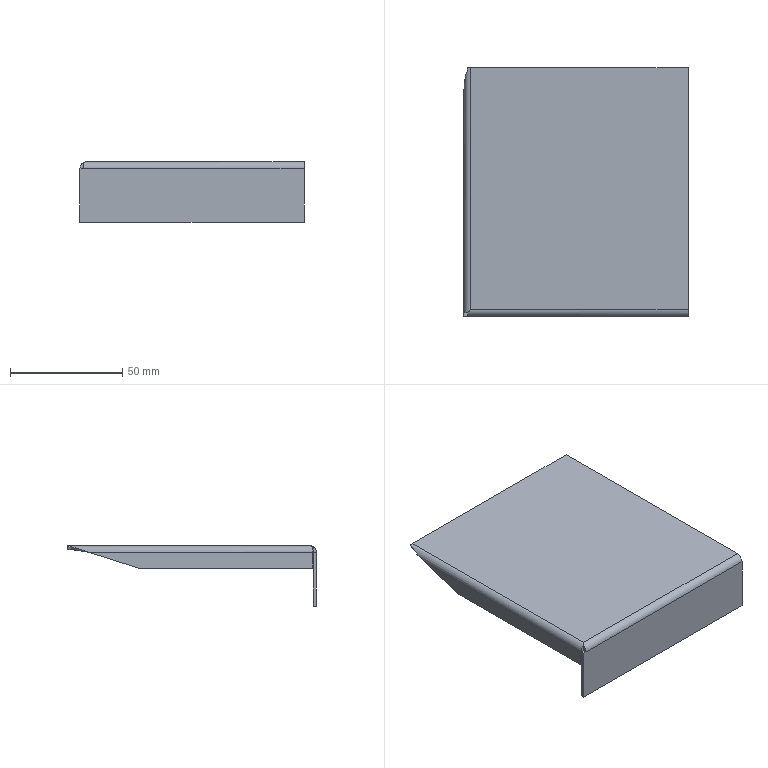Part | NX | features solid 2 | 1 solid | 23 faces | box 100 x 111 x 27 mm | volume 21325 mm3 | plane 18 | cylinder 4 | spline 1 | commonest cylinder face diameters 3 x2 6 x2
STEP:
#1=CARTESIAN_POINT('',(473.5,-28.4,8.5));
#2=VERTEX_POINT('',#1);
#3=CARTESIAN_POINT('',(473.5,71.235,8.5));
#4=VERTEX_POINT('',#3);
#5=CARTESIAN_POINT('',(473.5,-30.,8.5));
#6=DIRECTION('',(0.,1.,0.));
#7=VECTOR('',#6,1000.);
#8=LINE('',#5,#7);
#9=EDGE_CURVE('',#2,#4,#8,.T.);
#10=ORIENTED_EDGE('',*,*,#9,.T.);
#11=CARTESIAN_POINT('',(473.5,49.36,1.5));
#12=VERTEX_POINT('',#11);
#13=CARTESIAN_POINT('',(473.5,-19.726,-20.607));
#14=DIRECTION('',(0.,0.9524,0.3048));
#15=VECTOR('',#14,1000.);
#16=LINE('',#13,#15);
#17=EDGE_CURVE('',#12,#4,#16,.T.);
#18=ORIENTED_EDGE('',*,*,#17,.F.);
#19=CARTESIAN_POINT('',(473.5,-28.4,1.5));
#20=VERTEX_POINT('',#19);
#21=CARTESIAN_POINT('',(473.5,-30.,1.5));
#22=DIRECTION('',(0.,1.,0.));
#23=VECTOR('',#22,1000.);
#24=LINE('',#21,#23);
#25=EDGE_CURVE('',#20,#12,#24,.T.);
#26=ORIENTED_EDGE('',*,*,#25,.F.);
#27=CARTESIAN_POINT('',(473.5,-28.4,11.5));
#28=DIRECTION('',(0.,0.,-1.));
#29=VECTOR('',#28,1000.);
#30=LINE('',#27,#29);
#31=EDGE_CURVE('',#2,#20,#30,.T.);
#32=ORIENTED_EDGE('',*,*,#31,.F.);
#33=EDGE_LOOP('',(#10,#18,#26,#32));
#34=FACE_BOUND('',#33,.T.);
#35=CARTESIAN_POINT('',(473.5,-30.,11.5));
#36=DIRECTION('',(1.,0.,0.));
#37=DIRECTION('',(0.,1.,0.));
#38=AXIS2_PLACEMENT_3D('',#35,#36,#37);
#39=PLANE('',#38);
#40=ADVANCED_FACE('',(#34),#39,.F.);
#41=CARTESIAN_POINT('',(475.,49.36,1.5));
#42=VERTEX_POINT('',#41);
#43=CARTESIAN_POINT('',(475.,71.235,8.5));
#44=VERTEX_POINT('',#43);
#45=CARTESIAN_POINT('',(475.,-19.726,-20.607));
#46=DIRECTION('',(0.,0.9524,0.3048));
#47=VECTOR('',#46,1000.);
#48=LINE('',#45,#47);
#49=EDGE_CURVE('',#42,#44,#48,.T.);
#50=ORIENTED_EDGE('',*,*,#49,.T.);
#51=CARTESIAN_POINT('',(475.,-28.4,8.5));
#52=VERTEX_POINT('',#51);
#53=CARTESIAN_POINT('',(475.,-30.,8.5));
#54=DIRECTION('',(0.,1.,0.));
#55=VECTOR('',#54,1000.);
#56=LINE('',#53,#55);
#57=EDGE_CURVE('',#52,#44,#56,.T.);
#58=ORIENTED_EDGE('',*,*,#57,.F.);
#59=CARTESIAN_POINT('',(475.,-28.4,1.5));
#60=VERTEX_POINT('',#59);
#61=CARTESIAN_POINT('',(475.,-28.4,11.5));
#62=DIRECTION('',(0.,0.,-1.));
#63=VECTOR('',#62,1000.);
#64=LINE('',#61,#63);
#65=EDGE_CURVE('',#52,#60,#64,.T.);
#66=ORIENTED_EDGE('',*,*,#65,.T.);
#67=CARTESIAN_POINT('',(475.,-30.,1.5));
#68=DIRECTION('',(0.,1.,0.));
#69=VECTOR('',#68,1000.);
#70=LINE('',#67,#69);
#71=EDGE_CURVE('',#60,#42,#70,.T.);
#72=ORIENTED_EDGE('',*,*,#71,.T.);
#73=EDGE_LOOP('',(#50,#58,#66,#72));
#74=FACE_BOUND('',#73,.T.);
#75=CARTESIAN_POINT('',(475.,-30.,11.5));
#76=DIRECTION('',(1.,0.,0.));
#77=DIRECTION('',(0.,1.,0.));
#78=AXIS2_PLACEMENT_3D('',#75,#76,#77);
#79=PLANE('',#78);
#80=ADVANCED_FACE('',(#74),#79,.T.);
#81=CARTESIAN_POINT('',(473.5,49.36,1.5));
#82=DIRECTION('',(-1.,0.,0.));
#83=VECTOR('',#82,1000.);
#84=LINE('',#81,#83);
#85=EDGE_CURVE('',#42,#12,#84,.T.);
#86=ORIENTED_EDGE('',*,*,#85,.T.);
#87=ORIENTED_EDGE('',*,*,#17,.T.);
#88=CARTESIAN_POINT('',(473.5,71.235,8.5));
#89=DIRECTION('',(-1.,0.,0.));
#90=VECTOR('',#89,1000.);
#91=LINE('',#88,#90);
#92=EDGE_CURVE('',#44,#4,#91,.T.);
#93=ORIENTED_EDGE('',*,*,#92,.F.);
#94=ORIENTED_EDGE('',*,*,#49,.F.);
#95=EDGE_LOOP('',(#86,#87,#93,#94));
#96=FACE_BOUND('',#95,.T.);
#97=CARTESIAN_POINT('',(473.5,-19.726,-20.607));
#98=DIRECTION('',(0.,0.3048,-0.9524));
#99=DIRECTION('',(-1.,0.,0.));
#100=AXIS2_PLACEMENT_3D('',#97,#98,#99);
#101=PLANE('',#100);
#102=ADVANCED_FACE('',(#96),#101,.T.);
#103=ORIENTED_EDGE('',*,*,#85,.F.);
#104=ORIENTED_EDGE('',*,*,#71,.F.);
#105=CARTESIAN_POINT('',(473.5,-28.4,1.5));
#106=DIRECTION('',(-1.,0.,0.));
#107=VECTOR('',#106,1000.);
#108=LINE('',#105,#107);
#109=EDGE_CURVE('',#60,#20,#108,.T.);
#110=ORIENTED_EDGE('',*,*,#109,.T.);
#111=ORIENTED_EDGE('',*,*,#25,.T.);
#112=EDGE_LOOP('',(#103,#104,#110,#111));
#113=FACE_BOUND('',#112,.T.);
#114=CARTESIAN_POINT('',(473.5,-30.,1.5));
#115=DIRECTION('',(0.,0.,-1.));
#116=DIRECTION('',(0.,-1.,0.));
#117=AXIS2_PLACEMENT_3D('',#114,#115,#116);
#118=PLANE('',#117);
#119=ADVANCED_FACE('',(#113),#118,.T.);
#120=CARTESIAN_POINT('',(476.5,-27.,10.));
#121=VERTEX_POINT('',#120);
#122=CARTESIAN_POINT('',(573.5,-27.,10.));
#123=VERTEX_POINT('',#122);
#124=CARTESIAN_POINT('',(476.5,-27.,10.));
#125=DIRECTION('',(1.,0.,0.));
#126=VECTOR('',#125,1000.);
#127=LINE('',#124,#126);
#128=EDGE_CURVE('',#121,#123,#127,.T.);
#129=ORIENTED_EDGE('',*,*,#128,.F.);
#130=CARTESIAN_POINT('',(476.5,81.,10.));
#131=VERTEX_POINT('',#130);
#132=CARTESIAN_POINT('',(476.5,-30.,10.));
#133=DIRECTION('',(0.,1.,0.));
#134=VECTOR('',#133,1000.);
#135=LINE('',#132,#134);
#136=EDGE_CURVE('',#121,#131,#135,.T.);
#137=ORIENTED_EDGE('',*,*,#136,.T.);
#138=CARTESIAN_POINT('',(573.5,81.,10.));
#139=VERTEX_POINT('',#138);
#140=CARTESIAN_POINT('',(573.5,81.,10.));
#141=DIRECTION('',(-1.,0.,0.));
#142=VECTOR('',#141,1000.);
#143=LINE('',#140,#142);
#144=EDGE_CURVE('',#139,#131,#143,.T.);
#145=ORIENTED_EDGE('',*,*,#144,.F.);
#146=CARTESIAN_POINT('',(573.5,-30.,10.));
#147=DIRECTION('',(0.,1.,0.));
#148=VECTOR('',#147,1000.);
#149=LINE('',#146,#148);
#150=EDGE_CURVE('',#123,#139,#149,.T.);
#151=ORIENTED_EDGE('',*,*,#150,.F.);
#152=EDGE_LOOP('',(#129,#137,#145,#151));
#153=FACE_BOUND('',#152,.T.);
#154=CARTESIAN_POINT('',(573.5,-30.,10.));
#155=DIRECTION('',(0.,0.,-1.));
#156=DIRECTION('',(0.,-1.,0.));
#157=AXIS2_PLACEMENT_3D('',#154,#155,#156);
#158=PLANE('',#157);
#159=ADVANCED_FACE('',(#153),#158,.T.);
#160=CARTESIAN_POINT('',(476.5,-27.,11.5));
#161=VERTEX_POINT('',#160);
#162=CARTESIAN_POINT('',(476.5,81.,11.5));
#163=VERTEX_POINT('',#162);
#164=CARTESIAN_POINT('',(476.5,-30.,11.5));
#165=DIRECTION('',(0.,1.,0.));
#166=VECTOR('',#165,1000.);
#167=LINE('',#164,#166);
#168=EDGE_CURVE('',#161,#163,#167,.T.);
#169=ORIENTED_EDGE('',*,*,#168,.F.);
#170=CARTESIAN_POINT('',(573.5,-27.,11.5));
#171=VERTEX_POINT('',#170);
#172=CARTESIAN_POINT('',(476.5,-27.,11.5));
#173=DIRECTION('',(1.,0.,0.));
#174=VECTOR('',#173,1000.);
#175=LINE('',#172,#174);
#176=EDGE_CURVE('',#161,#171,#175,.T.);
#177=ORIENTED_EDGE('',*,*,#176,.T.);
#178=CARTESIAN_POINT('',(573.5,81.,11.5));
#179=VERTEX_POINT('',#178);
#180=CARTESIAN_POINT('',(573.5,-30.,11.5));
#181=DIRECTION('',(0.,1.,0.));
#182=VECTOR('',#181,1000.);
#183=LINE('',#180,#182);
#184=EDGE_CURVE('',#171,#179,#183,.T.);
#185=ORIENTED_EDGE('',*,*,#184,.T.);
#186=CARTESIAN_POINT('',(573.5,81.,11.5));
#187=DIRECTION('',(-1.,0.,0.));
#188=VECTOR('',#187,1000.);
#189=LINE('',#186,#188);
#190=EDGE_CURVE('',#179,#163,#189,.T.);
#191=ORIENTED_EDGE('',*,*,#190,.T.);
#192=EDGE_LOOP('',(#169,#177,#185,#191));
#193=FACE_BOUND('',#192,.T.);
#194=CARTESIAN_POINT('',(573.5,-30.,11.5));
#195=DIRECTION('',(0.,0.,-1.));
#196=DIRECTION('',(0.,-1.,0.));
#197=AXIS2_PLACEMENT_3D('',#194,#195,#196);
#198=PLANE('',#197);
#199=ADVANCED_FACE('',(#193),#198,.F.);
#200=CARTESIAN_POINT('',(475.1,-30.,8.5));
#201=VERTEX_POINT('',#200);
#202=CARTESIAN_POINT('',(475.1,-28.5,8.5));
#203=VERTEX_POINT('',#202);
#204=CARTESIAN_POINT('',(475.1,-30.,8.5));
#205=DIRECTION('',(0.,1.,0.));
#206=VECTOR('',#205,1000.);
#207=LINE('',#204,#206);
#208=EDGE_CURVE('',#201,#203,#207,.T.);
#209=ORIENTED_EDGE('',*,*,#208,.F.);
#210=CARTESIAN_POINT('',(475.1,-28.5,11.098));
#211=VERTEX_POINT('',#210);
#212=CARTESIAN_POINT('',(475.1,-27.,8.5));
#213=DIRECTION('',(-1.,0.,0.));
#214=DIRECTION('',(0.,0.,1.));
#215=AXIS2_PLACEMENT_3D('',#212,#213,#214);
#216=CIRCLE('',#215,3.);
#217=EDGE_CURVE('',#201,#211,#216,.T.);
#218=ORIENTED_EDGE('',*,*,#217,.T.);
#219=CARTESIAN_POINT('',(475.1,-28.5,-988.5));
#220=DIRECTION('',(0.,0.,-1.));
#221=VECTOR('',#220,1000.);
#222=LINE('',#219,#221);
#223=EDGE_CURVE('',#211,#203,#222,.T.);
#224=ORIENTED_EDGE('',*,*,#223,.T.);
#225=EDGE_LOOP('',(#209,#218,#224));
#226=FACE_BOUND('',#225,.T.);
#227=CARTESIAN_POINT('',(475.1,-28.5,1011.5));
#228=DIRECTION('',(1.,0.,0.));
#229=DIRECTION('',(0.,1.,0.));
#230=AXIS2_PLACEMENT_3D('',#227,#228,#229);
#231=PLANE('',#230);
#232=ADVANCED_FACE('',(#226),#231,.F.);
#233=CARTESIAN_POINT('',(475.1,-28.5,8.5));
#234=CARTESIAN_POINT('',(475.1,-28.5,9.379));
#235=CARTESIAN_POINT('',(475.68,-27.879,10.));
#236=CARTESIAN_POINT('',(476.5,-27.,10.));
#237=(BOUNDED_CURVE()B_SPLINE_CURVE(3,(#233,#234,#235,#236),.UNSPECIFIED.,.F.,.F.)B_SPLINE_CURVE_WITH_KNOTS((4,4),(3.142,4.712),.PIECEWISE_BEZIER_KNOTS.)CURVE()GEOMETRIC_REPRESENTATION_ITEM()RATIONAL_B_SPLINE_CURVE((1.,0.8047,0.8047,1.))REPRESENTATION_ITEM(''));
#238=EDGE_CURVE('',#203,#121,#237,.T.);
#239=ORIENTED_EDGE('',*,*,#238,.F.);
#240=ORIENTED_EDGE('',*,*,#223,.F.);
#241=CARTESIAN_POINT('',(475.1,-28.5,11.098));
#242=CARTESIAN_POINT('',(475.528,-28.041,11.363));
#243=CARTESIAN_POINT('',(476.006,-27.53,11.5));
#244=CARTESIAN_POINT('',(476.5,-27.,11.5));
#245=(BOUNDED_CURVE()B_SPLINE_CURVE(3,(#241,#242,#243,#244),.UNSPECIFIED.,.F.,.F.)B_SPLINE_CURVE_WITH_KNOTS((4,4),(4.189,4.712),.PIECEWISE_BEZIER_KNOTS.)CURVE()GEOMETRIC_REPRESENTATION_ITEM()RATIONAL_B_SPLINE_CURVE((1.,0.9773,0.9773,1.))REPRESENTATION_ITEM(''));
#246=EDGE_CURVE('',#211,#161,#245,.T.);
#247=ORIENTED_EDGE('',*,*,#246,.T.);
#248=CARTESIAN_POINT('',(476.5,-27.,10.));
#249=DIRECTION('',(0.,0.,1.));
#250=VECTOR('',#249,1000.);
#251=LINE('',#248,#250);
#252=EDGE_CURVE('',#121,#161,#251,.T.);
#253=ORIENTED_EDGE('',*,*,#252,.F.);
#254=EDGE_LOOP('',(#239,#240,#247,#253));
#255=FACE_BOUND('',#254,.T.);
#256=CARTESIAN_POINT('',(1158.818,704.055,1011.5));
#257=DIRECTION('',(0.7311,-0.6823,0.));
#258=DIRECTION('',(0.,0.,-1.));
#259=AXIS2_PLACEMENT_3D('',#256,#257,#258);
#260=PLANE('',#259);
#261=ADVANCED_FACE('',(#255),#260,.F.);
#262=ORIENTED_EDGE('',*,*,#246,.F.);
#263=ORIENTED_EDGE('',*,*,#217,.F.);
#264=CARTESIAN_POINT('',(573.5,-30.,8.5));
#265=VERTEX_POINT('',#264);
#266=CARTESIAN_POINT('',(573.5,-30.,8.5));
#267=DIRECTION('',(-1.,0.,0.));
#268=VECTOR('',#267,1000.);
#269=LINE('',#266,#268);
#270=EDGE_CURVE('',#265,#201,#269,.T.);
#271=ORIENTED_EDGE('',*,*,#270,.F.);
#272=CARTESIAN_POINT('',(573.5,-27.,8.5));
#273=DIRECTION('',(-1.,0.,0.));
#274=DIRECTION('',(0.,0.,-1.));
#275=AXIS2_PLACEMENT_3D('',#272,#273,#274);
#276=CIRCLE('',#275,3.);
#277=EDGE_CURVE('',#265,#171,#276,.T.);
#278=ORIENTED_EDGE('',*,*,#277,.T.);
#279=ORIENTED_EDGE('',*,*,#176,.F.);
#280=EDGE_LOOP('',(#262,#263,#271,#278,#279));
#281=FACE_BOUND('',#280,.T.);
#282=CARTESIAN_POINT('',(476.5,-27.,8.5));
#283=DIRECTION('',(1.,0.,0.));
#284=DIRECTION('',(0.,0.,-1.));
#285=AXIS2_PLACEMENT_3D('',#282,#283,#284);
#286=CYLINDRICAL_SURFACE('',#285,3.);
#287=ADVANCED_FACE('',(#281),#286,.T.);
#288=ORIENTED_EDGE('',*,*,#277,.F.);
#289=CARTESIAN_POINT('',(573.5,-30.,-15.5));
#290=VERTEX_POINT('',#289);
#291=CARTESIAN_POINT('',(573.5,-30.,10.208));
#292=DIRECTION('',(0.,0.,1.));
#293=VECTOR('',#292,1000.);
#294=LINE('',#291,#293);
#295=EDGE_CURVE('',#290,#265,#294,.T.);
#296=ORIENTED_EDGE('',*,*,#295,.F.);
#297=CARTESIAN_POINT('',(573.5,-28.5,-15.5));
#298=VERTEX_POINT('',#297);
#299=CARTESIAN_POINT('',(573.5,-30.,-15.5));
#300=DIRECTION('',(0.,1.,0.));
#301=VECTOR('',#300,1000.);
#302=LINE('',#299,#301);
#303=EDGE_CURVE('',#290,#298,#302,.T.);
#304=ORIENTED_EDGE('',*,*,#303,.T.);
#305=CARTESIAN_POINT('',(573.5,-28.5,8.5));
#306=VERTEX_POINT('',#305);
#307=CARTESIAN_POINT('',(573.5,-28.5,10.208));
#308=DIRECTION('',(0.,0.,1.));
#309=VECTOR('',#308,1000.);
#310=LINE('',#307,#309);
#311=EDGE_CURVE('',#298,#306,#310,.T.);
#312=ORIENTED_EDGE('',*,*,#311,.T.);
#313=CARTESIAN_POINT('',(573.5,-27.,8.5));
#314=DIRECTION('',(-1.,0.,0.));
#315=DIRECTION('',(0.,0.,1.));
#316=AXIS2_PLACEMENT_3D('',#313,#314,#315);
#317=CIRCLE('',#316,1.5);
#318=EDGE_CURVE('',#306,#123,#317,.T.);
#319=ORIENTED_EDGE('',*,*,#318,.T.);
#320=ORIENTED_EDGE('',*,*,#150,.T.);
#321=CARTESIAN_POINT('',(573.5,81.,11.5));
#322=DIRECTION('',(0.,0.,1.));
#323=VECTOR('',#322,1000.);
#324=LINE('',#321,#323);
#325=EDGE_CURVE('',#139,#179,#324,.T.);
#326=ORIENTED_EDGE('',*,*,#325,.T.);
#327=ORIENTED_EDGE('',*,*,#184,.F.);
#328=EDGE_LOOP('',(#288,#296,#304,#312,#319,#320,#326,#327));
#329=FACE_BOUND('',#328,.T.);
#330=CARTESIAN_POINT('',(573.5,-30.,11.5));
#331=DIRECTION('',(-1.,0.,0.));
#332=DIRECTION('',(0.,1.,0.));
#333=AXIS2_PLACEMENT_3D('',#330,#331,#332);
#334=PLANE('',#333);
#335=ADVANCED_FACE('',(#329),#334,.F.);
#336=CARTESIAN_POINT('',(573.5,-28.5,8.5));
#337=DIRECTION('',(-1.,0.,0.));
#338=VECTOR('',#337,1000.);
#339=LINE('',#336,#338);
#340=EDGE_CURVE('',#306,#203,#339,.T.);
#341=ORIENTED_EDGE('',*,*,#340,.T.);
#342=ORIENTED_EDGE('',*,*,#238,.T.);
#343=ORIENTED_EDGE('',*,*,#128,.T.);
#344=ORIENTED_EDGE('',*,*,#318,.F.);
#345=EDGE_LOOP('',(#341,#342,#343,#344));
#346=FACE_BOUND('',#345,.T.);
#347=CARTESIAN_POINT('',(476.5,-27.,8.5));
#348=DIRECTION('',(1.,0.,0.));
#349=DIRECTION('',(0.,0.,-1.));
#350=AXIS2_PLACEMENT_3D('',#347,#348,#349);
#351=CYLINDRICAL_SURFACE('',#350,1.5);
#352=ADVANCED_FACE('',(#346),#351,.F.);
#353=CARTESIAN_POINT('',(476.5,-27.,10.));
#354=CARTESIAN_POINT('',(475.621,-27.82,10.));
#355=CARTESIAN_POINT('',(475.,-28.4,9.379));
#356=CARTESIAN_POINT('',(475.,-28.4,8.5));
#357=(BOUNDED_CURVE()B_SPLINE_CURVE(3,(#353,#354,#355,#356),.UNSPECIFIED.,.F.,.F.)B_SPLINE_CURVE_WITH_KNOTS((4,4),(1.571,3.142),.PIECEWISE_BEZIER_KNOTS.)CURVE()GEOMETRIC_REPRESENTATION_ITEM()RATIONAL_B_SPLINE_CURVE((1.,0.8047,0.8047,1.))REPRESENTATION_ITEM(''));
#358=EDGE_CURVE('',#121,#52,#357,.T.);
#359=ORIENTED_EDGE('',*,*,#358,.F.);
#360=ORIENTED_EDGE('',*,*,#252,.T.);
#361=CARTESIAN_POINT('',(475.,-28.4,11.098));
#362=VERTEX_POINT('',#361);
#363=CARTESIAN_POINT('',(476.5,-27.,11.5));
#364=CARTESIAN_POINT('',(475.97,-27.494,11.5));
#365=CARTESIAN_POINT('',(475.459,-27.972,11.363));
#366=CARTESIAN_POINT('',(475.,-28.4,11.098));
#367=(BOUNDED_CURVE()B_SPLINE_CURVE(3,(#363,#364,#365,#366),.UNSPECIFIED.,.F.,.F.)B_SPLINE_CURVE_WITH_KNOTS((4,4),(1.571,2.094),.PIECEWISE_BEZIER_KNOTS.)CURVE()GEOMETRIC_REPRESENTATION_ITEM()RATIONAL_B_SPLINE_CURVE((1.,0.9773,0.9773,1.))REPRESENTATION_ITEM(''));
#368=EDGE_CURVE('',#161,#362,#367,.T.);
#369=ORIENTED_EDGE('',*,*,#368,.T.);
#370=CARTESIAN_POINT('',(475.,-28.4,-988.5));
#371=DIRECTION('',(0.,0.,-1.));
#372=VECTOR('',#371,1000.);
#373=LINE('',#370,#372);
#374=EDGE_CURVE('',#362,#52,#373,.T.);
#375=ORIENTED_EDGE('',*,*,#374,.T.);
#376=EDGE_LOOP('',(#359,#360,#369,#375));
#377=FACE_BOUND('',#376,.T.);
#378=CARTESIAN_POINT('',(1207.555,655.318,1011.5));
#379=DIRECTION('',(0.6823,-0.7311,0.));
#380=DIRECTION('',(0.,0.,-1.));
#381=AXIS2_PLACEMENT_3D('',#378,#379,#380);
#382=PLANE('',#381);
#383=ADVANCED_FACE('',(#377),#382,.T.);
#384=CARTESIAN_POINT('',(476.5,-28.4,8.5));
#385=DIRECTION('',(0.,-1.,0.));
#386=DIRECTION('',(0.,0.,-1.));
#387=AXIS2_PLACEMENT_3D('',#384,#385,#386);
#388=CIRCLE('',#387,3.);
#389=EDGE_CURVE('',#362,#2,#388,.T.);
#390=ORIENTED_EDGE('',*,*,#389,.T.);
#391=ORIENTED_EDGE('',*,*,#31,.T.);
#392=ORIENTED_EDGE('',*,*,#109,.F.);
#393=ORIENTED_EDGE('',*,*,#65,.F.);
#394=ORIENTED_EDGE('',*,*,#374,.F.);
#395=EDGE_LOOP('',(#390,#391,#392,#393,#394));
#396=FACE_BOUND('',#395,.T.);
#397=CARTESIAN_POINT('',(475.,-28.4,1011.5));
#398=DIRECTION('',(0.,-1.,0.));
#399=DIRECTION('',(-1.,0.,0.));
#400=AXIS2_PLACEMENT_3D('',#397,#398,#399);
#401=PLANE('',#400);
#402=ADVANCED_FACE('',(#396),#401,.T.);
#403=CARTESIAN_POINT('',(475.75,81.,9.799));
#404=VERTEX_POINT('',#403);
#405=CARTESIAN_POINT('',(475.75,79.354,9.799));
#406=VERTEX_POINT('',#405);
#407=CARTESIAN_POINT('',(475.75,-30.,9.799));
#408=DIRECTION('',(0.,-1.,0.));
#409=VECTOR('',#408,1000.);
#410=LINE('',#407,#409);
#411=EDGE_CURVE('',#404,#406,#410,.T.);
#412=ORIENTED_EDGE('',*,*,#411,.T.);
#413=CARTESIAN_POINT('',(475.,79.354,11.098));
#414=VERTEX_POINT('',#413);
#415=CARTESIAN_POINT('',(475.,79.354,11.098));
#416=DIRECTION('',(-0.5,0.,0.866));
#417=VECTOR('',#416,1000.);
#418=LINE('',#415,#417);
#419=EDGE_CURVE('',#406,#414,#418,.T.);
#420=ORIENTED_EDGE('',*,*,#419,.T.);
#421=CARTESIAN_POINT('',(475.,81.,11.098));
#422=VERTEX_POINT('',#421);
#423=CARTESIAN_POINT('',(475.,-30.,11.098));
#424=DIRECTION('',(0.,-1.,0.));
#425=VECTOR('',#424,1000.);
#426=LINE('',#423,#425);
#427=EDGE_CURVE('',#422,#414,#426,.T.);
#428=ORIENTED_EDGE('',*,*,#427,.F.);
#429=CARTESIAN_POINT('',(475.,81.,11.098));
#430=DIRECTION('',(-0.5,0.,0.866));
#431=VECTOR('',#430,1000.);
#432=LINE('',#429,#431);
#433=EDGE_CURVE('',#404,#422,#432,.T.);
#434=ORIENTED_EDGE('',*,*,#433,.F.);
#435=EDGE_LOOP('',(#412,#420,#428,#434));
#436=FACE_BOUND('',#435,.T.);
#437=CARTESIAN_POINT('',(475.,80.177,11.098));
#438=DIRECTION('',(0.866,0.,0.5));
#439=DIRECTION('',(0.,-1.,0.));
#440=AXIS2_PLACEMENT_3D('',#437,#438,#439);
#441=PLANE('',#440);
#442=ADVANCED_FACE('',(#436),#441,.F.);
#443=ORIENTED_EDGE('',*,*,#92,.T.);
#444=CARTESIAN_POINT('',(473.5,71.235,8.5));
#445=CARTESIAN_POINT('',(473.5,74.666,9.598));
#446=CARTESIAN_POINT('',(474.049,77.638,10.549));
#447=CARTESIAN_POINT('',(475.,79.354,11.098));
#448=(BOUNDED_CURVE()B_SPLINE_CURVE(3,(#444,#445,#446,#447),.UNSPECIFIED.,.F.,.F.)B_SPLINE_CURVE_WITH_KNOTS((4,4),(4.712,5.76),.PIECEWISE_BEZIER_KNOTS.)CURVE()GEOMETRIC_REPRESENTATION_ITEM()RATIONAL_B_SPLINE_CURVE((1.,0.9107,0.9107,1.))REPRESENTATION_ITEM(''));
#449=EDGE_CURVE('',#4,#414,#448,.T.);
#450=ORIENTED_EDGE('',*,*,#449,.T.);
#451=ORIENTED_EDGE('',*,*,#419,.F.);
#452=CARTESIAN_POINT('',(475.,71.235,8.5));
#453=CARTESIAN_POINT('',(475.,74.666,9.049));
#454=CARTESIAN_POINT('',(475.275,77.638,9.525));
#455=CARTESIAN_POINT('',(475.75,79.354,9.799));
#456=(BOUNDED_CURVE()B_SPLINE_CURVE(3,(#452,#453,#454,#455),.UNSPECIFIED.,.F.,.F.)B_SPLINE_CURVE_WITH_KNOTS((4,4),(4.712,5.76),.PIECEWISE_BEZIER_KNOTS.)CURVE()GEOMETRIC_REPRESENTATION_ITEM()RATIONAL_B_SPLINE_CURVE((1.,0.9107,0.9107,1.))REPRESENTATION_ITEM(''));
#457=EDGE_CURVE('',#44,#406,#456,.T.);
#458=ORIENTED_EDGE('',*,*,#457,.F.);
#459=EDGE_LOOP('',(#443,#450,#451,#458));
#460=FACE_BOUND('',#459,.T.);
#461=CARTESIAN_POINT('',(475.,71.235,8.5));
#462=CARTESIAN_POINT('',(474.5,71.235,8.5));
#463=CARTESIAN_POINT('',(474.,71.235,8.5));
#464=CARTESIAN_POINT('',(473.5,71.235,8.5));
#465=CARTESIAN_POINT('',(475.,74.843,9.077));
#466=CARTESIAN_POINT('',(474.5,74.843,9.27));
#467=CARTESIAN_POINT('',(474.,74.843,9.462));
#468=CARTESIAN_POINT('',(473.5,74.843,9.655));
#469=CARTESIAN_POINT('',(475.3,77.73,9.539));
#470=CARTESIAN_POINT('',(474.9,77.73,9.886));
#471=CARTESIAN_POINT('',(474.5,77.73,10.232));
#472=CARTESIAN_POINT('',(474.1,77.73,10.578));
#473=CARTESIAN_POINT('',(475.75,79.354,9.799));
#474=CARTESIAN_POINT('',(475.5,79.354,10.232));
#475=CARTESIAN_POINT('',(475.25,79.354,10.665));
#476=CARTESIAN_POINT('',(475.,79.354,11.098));
#477=(BOUNDED_SURFACE()B_SPLINE_SURFACE(3,3,((#461,#462,#463,#464),(#465,#466,#467,#468),(#469,#470,#471,#472),(#473,#474,#475,#476)),.UNSPECIFIED.,.F.,.F.,.F.)B_SPLINE_SURFACE_WITH_KNOTS((4,4),(4,4),(0.75,0.8943),(0.,1.),.PIECEWISE_BEZIER_KNOTS.)GEOMETRIC_REPRESENTATION_ITEM()RATIONAL_B_SPLINE_SURFACE(((0.5,0.5,0.5,0.5),(0.5,0.5,0.5,0.5),(0.5556,0.5556,0.5556,0.5556),(0.6667,0.6667,0.6667,0.6667)))REPRESENTATION_ITEM('')SURFACE());
#478=ADVANCED_FACE('',(#460),#477,.F.);
#479=CARTESIAN_POINT('',(476.5,81.,8.5));
#480=DIRECTION('',(0.,-1.,0.));
#481=DIRECTION('',(-1.,0.,0.));
#482=AXIS2_PLACEMENT_3D('',#479,#480,#481);
#483=CIRCLE('',#482,3.);
#484=EDGE_CURVE('',#163,#422,#483,.T.);
#485=ORIENTED_EDGE('',*,*,#484,.F.);
#486=ORIENTED_EDGE('',*,*,#190,.F.);
#487=ORIENTED_EDGE('',*,*,#325,.F.);
#488=ORIENTED_EDGE('',*,*,#144,.T.);
#489=CARTESIAN_POINT('',(476.5,81.,8.5));
#490=DIRECTION('',(0.,-1.,0.));
#491=DIRECTION('',(0.,0.,1.));
#492=AXIS2_PLACEMENT_3D('',#489,#490,#491);
#493=CIRCLE('',#492,1.5);
#494=EDGE_CURVE('',#131,#404,#493,.T.);
#495=ORIENTED_EDGE('',*,*,#494,.T.);
#496=ORIENTED_EDGE('',*,*,#433,.T.);
#497=EDGE_LOOP('',(#485,#486,#487,#488,#495,#496));
#498=FACE_BOUND('',#497,.T.);
#499=CARTESIAN_POINT('',(476.5,81.,8.5));
#500=DIRECTION('',(0.,-1.,0.));
#501=DIRECTION('',(-1.,0.,0.));
#502=AXIS2_PLACEMENT_3D('',#499,#500,#501);
#503=PLANE('',#502);
#504=ADVANCED_FACE('',(#498),#503,.F.);
#505=ORIENTED_EDGE('',*,*,#368,.F.);
#506=ORIENTED_EDGE('',*,*,#168,.T.);
#507=ORIENTED_EDGE('',*,*,#484,.T.);
#508=ORIENTED_EDGE('',*,*,#427,.T.);
#509=ORIENTED_EDGE('',*,*,#449,.F.);
#510=ORIENTED_EDGE('',*,*,#9,.F.);
#511=ORIENTED_EDGE('',*,*,#389,.F.);
#512=EDGE_LOOP('',(#505,#506,#507,#508,#509,#510,#511));
#513=FACE_BOUND('',#512,.T.);
#514=CARTESIAN_POINT('',(476.5,-30.,8.5));
#515=DIRECTION('',(0.,1.,0.));
#516=DIRECTION('',(0.,0.,1.));
#517=AXIS2_PLACEMENT_3D('',#514,#515,#516);
#518=CYLINDRICAL_SURFACE('',#517,3.);
#519=ADVANCED_FACE('',(#513),#518,.T.);
#520=ORIENTED_EDGE('',*,*,#136,.F.);
#521=ORIENTED_EDGE('',*,*,#358,.T.);
#522=ORIENTED_EDGE('',*,*,#57,.T.);
#523=ORIENTED_EDGE('',*,*,#457,.T.);
#524=ORIENTED_EDGE('',*,*,#411,.F.);
#525=ORIENTED_EDGE('',*,*,#494,.F.);
#526=EDGE_LOOP('',(#520,#521,#522,#523,#524,#525));
#527=FACE_BOUND('',#526,.T.);
#528=CARTESIAN_POINT('',(476.5,-30.,8.5));
#529=DIRECTION('',(0.,1.,0.));
#530=DIRECTION('',(0.,0.,1.));
#531=AXIS2_PLACEMENT_3D('',#528,#529,#530);
#532=CYLINDRICAL_SURFACE('',#531,1.5);
#533=ADVANCED_FACE('',(#527),#532,.F.);
#534=ORIENTED_EDGE('',*,*,#295,.T.);
#535=ORIENTED_EDGE('',*,*,#270,.T.);
#536=CARTESIAN_POINT('',(473.5,-30.,8.5));
#537=VERTEX_POINT('',#536);
#538=CARTESIAN_POINT('',(573.5,-30.,8.5));
#539=DIRECTION('',(-1.,0.,0.));
#540=VECTOR('',#539,1000.);
#541=LINE('',#538,#540);
#542=EDGE_CURVE('',#201,#537,#541,.T.);
#543=ORIENTED_EDGE('',*,*,#542,.T.);
#544=CARTESIAN_POINT('',(473.5,-30.,-15.5));
#545=VERTEX_POINT('',#544);
#546=CARTESIAN_POINT('',(473.5,-30.,10.208));
#547=DIRECTION('',(0.,0.,-1.));
#548=VECTOR('',#547,1000.);
#549=LINE('',#546,#548);
#550=EDGE_CURVE('',#537,#545,#549,.T.);
#551=ORIENTED_EDGE('',*,*,#550,.T.);
#552=CARTESIAN_POINT('',(476.5,-30.,-15.5));
#553=DIRECTION('',(1.,0.,0.));
#554=VECTOR('',#553,1000.);
#555=LINE('',#552,#554);
#556=EDGE_CURVE('',#545,#290,#555,.T.);
#557=ORIENTED_EDGE('',*,*,#556,.T.);
#558=EDGE_LOOP('',(#534,#535,#543,#551,#557));
#559=FACE_BOUND('',#558,.T.);
#560=CARTESIAN_POINT('',(523.5,-30.,6.5));
#561=DIRECTION('',(0.,-1.,0.));
#562=DIRECTION('',(-1.,0.,0.));
#563=AXIS2_PLACEMENT_3D('',#560,#561,#562);
#564=PLANE('',#563);
#565=ADVANCED_FACE('',(#559),#564,.T.);
#566=ORIENTED_EDGE('',*,*,#340,.F.);
#567=ORIENTED_EDGE('',*,*,#311,.F.);
#568=CARTESIAN_POINT('',(473.5,-28.5,-15.5));
#569=VERTEX_POINT('',#568);
#570=CARTESIAN_POINT('',(476.5,-28.5,-15.5));
#571=DIRECTION('',(1.,0.,0.));
#572=VECTOR('',#571,1000.);
#573=LINE('',#570,#572);
#574=EDGE_CURVE('',#569,#298,#573,.T.);
#575=ORIENTED_EDGE('',*,*,#574,.F.);
#576=CARTESIAN_POINT('',(473.5,-28.5,8.5));
#577=VERTEX_POINT('',#576);
#578=CARTESIAN_POINT('',(473.5,-28.5,10.208));
#579=DIRECTION('',(0.,0.,-1.));
#580=VECTOR('',#579,1000.);
#581=LINE('',#578,#580);
#582=EDGE_CURVE('',#577,#569,#581,.T.);
#583=ORIENTED_EDGE('',*,*,#582,.F.);
#584=CARTESIAN_POINT('',(573.5,-28.5,8.5));
#585=DIRECTION('',(-1.,0.,0.));
#586=VECTOR('',#585,1000.);
#587=LINE('',#584,#586);
#588=EDGE_CURVE('',#203,#577,#587,.T.);
#589=ORIENTED_EDGE('',*,*,#588,.F.);
#590=EDGE_LOOP('',(#566,#567,#575,#583,#589));
#591=FACE_BOUND('',#590,.T.);
#592=CARTESIAN_POINT('',(523.5,-28.5,6.5));
#593=DIRECTION('',(0.,-1.,0.));
#594=DIRECTION('',(-1.,0.,0.));
#595=AXIS2_PLACEMENT_3D('',#592,#593,#594);
#596=PLANE('',#595);
#597=ADVANCED_FACE('',(#591),#596,.F.);
#598=ORIENTED_EDGE('',*,*,#550,.F.);
#599=CARTESIAN_POINT('',(473.5,-30.,8.5));
#600=DIRECTION('',(0.,1.,0.));
#601=VECTOR('',#600,1000.);
#602=LINE('',#599,#601);
#603=EDGE_CURVE('',#537,#577,#602,.T.);
#604=ORIENTED_EDGE('',*,*,#603,.T.);
#605=ORIENTED_EDGE('',*,*,#582,.T.);
#606=CARTESIAN_POINT('',(473.5,-30.,-15.5));
#607=DIRECTION('',(0.,1.,0.));
#608=VECTOR('',#607,1000.);
#609=LINE('',#606,#608);
#610=EDGE_CURVE('',#545,#569,#609,.T.);
#611=ORIENTED_EDGE('',*,*,#610,.F.);
#612=EDGE_LOOP('',(#598,#604,#605,#611));
#613=FACE_BOUND('',#612,.T.);
#614=CARTESIAN_POINT('',(473.5,-30.,10.208));
#615=DIRECTION('',(1.,0.,0.));
#616=DIRECTION('',(0.,1.,0.));
#617=AXIS2_PLACEMENT_3D('',#614,#615,#616);
#618=PLANE('',#617);
#619=ADVANCED_FACE('',(#613),#618,.F.);
#620=ORIENTED_EDGE('',*,*,#574,.T.);
#621=ORIENTED_EDGE('',*,*,#303,.F.);
#622=ORIENTED_EDGE('',*,*,#556,.F.);
#623=ORIENTED_EDGE('',*,*,#610,.T.);
#624=EDGE_LOOP('',(#620,#621,#622,#623));
#625=FACE_BOUND('',#624,.T.);
#626=CARTESIAN_POINT('',(476.5,-30.,-15.5));
#627=DIRECTION('',(0.,0.,1.));
#628=DIRECTION('',(0.,-1.,0.));
#629=AXIS2_PLACEMENT_3D('',#626,#627,#628);
#630=PLANE('',#629);
#631=ADVANCED_FACE('',(#625),#630,.F.);
#632=ORIENTED_EDGE('',*,*,#542,.F.);
#633=ORIENTED_EDGE('',*,*,#208,.T.);
#634=ORIENTED_EDGE('',*,*,#588,.T.);
#635=ORIENTED_EDGE('',*,*,#603,.F.);
#636=EDGE_LOOP('',(#632,#633,#634,#635));
#637=FACE_BOUND('',#636,.T.);
#638=CARTESIAN_POINT('',(523.5,-30.,8.5));
#639=DIRECTION('',(0.,0.,1.));
#640=DIRECTION('',(0.,-1.,0.));
#641=AXIS2_PLACEMENT_3D('',#638,#639,#640);
#642=PLANE('',#641);
#643=ADVANCED_FACE('',(#637),#642,.T.);
#644=CLOSED_SHELL('',(#40,#80,#102,#119,#159,#199,#232,#261,#287,#335,#352,#383,#402,#442,#478,#504,#519,#533,#565,#597,#619,#631,#643));
#645=MANIFOLD_SOLID_BREP('',#644);
#646=(LENGTH_UNIT()NAMED_UNIT(*)SI_UNIT(.MILLI.,.METRE.));
#647=UNCERTAINTY_MEASURE_WITH_UNIT(LENGTH_MEASURE(0.00001),#646,'','');
#648=(NAMED_UNIT(*)PLANE_ANGLE_UNIT()SI_UNIT($,.RADIAN.));
#649=(NAMED_UNIT(*)SI_UNIT($,.STERADIAN.)SOLID_ANGLE_UNIT());
#650=(GEOMETRIC_REPRESENTATION_CONTEXT(3)GLOBAL_UNCERTAINTY_ASSIGNED_CONTEXT((#647))GLOBAL_UNIT_ASSIGNED_CONTEXT((#646,#648,#649))REPRESENTATION_CONTEXT('',''));
#651=ADVANCED_BREP_SHAPE_REPRESENTATION('',(#645),#650);